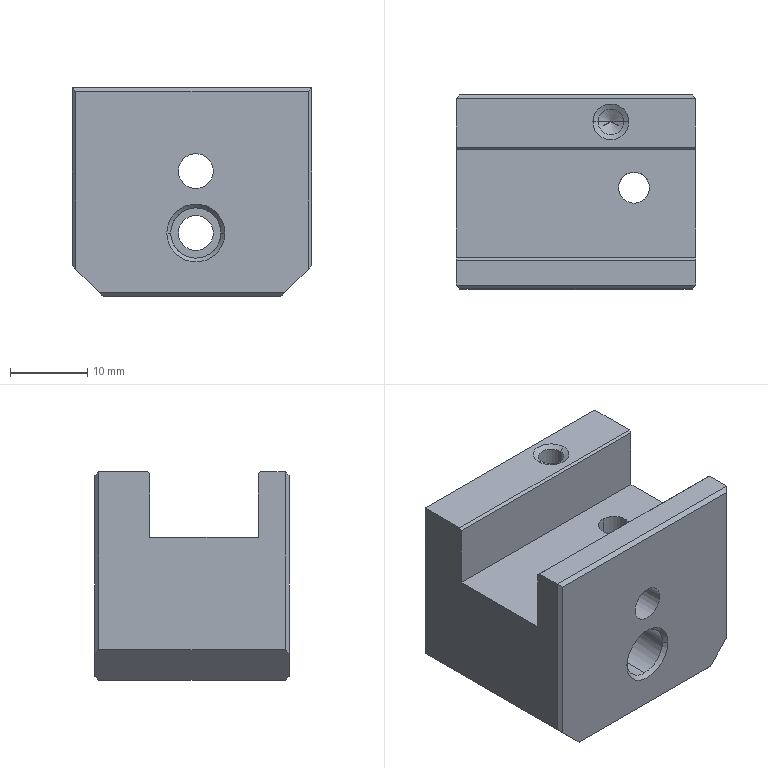Part | NX | 1 solid | 51 faces | box 31 x 25.1 x 27 mm | volume 15480 mm3 | plane 23 | cone 14 | cylinder 14 | commonest cylinder face diameters 3.3 x6 4.5 x4 4 x2 6.5 x2
STEP:
#1=CARTESIAN_POINT('',(29.,6.2,0.));
#2=VERTEX_POINT('',#1);
#3=CARTESIAN_POINT('',(-2.,6.2,0.));
#4=VERTEX_POINT('',#3);
#5=CARTESIAN_POINT('',(0.,6.2,0.));
#6=DIRECTION('',(-1.,0.,0.));
#7=VECTOR('',#6,1000.);
#8=LINE('',#5,#7);
#9=EDGE_CURVE('',#2,#4,#8,.T.);
#10=ORIENTED_EDGE('',*,*,#9,.T.);
#11=CARTESIAN_POINT('',(-2.,3.,0.));
#12=VERTEX_POINT('',#11);
#13=CARTESIAN_POINT('',(-2.,0.,0.));
#14=DIRECTION('',(0.,1.,0.));
#15=VECTOR('',#14,1000.);
#16=LINE('',#13,#15);
#17=EDGE_CURVE('',#12,#4,#16,.T.);
#18=ORIENTED_EDGE('',*,*,#17,.F.);
#19=CARTESIAN_POINT('',(29.,3.,0.));
#20=VERTEX_POINT('',#19);
#21=CARTESIAN_POINT('',(0.,3.,0.));
#22=DIRECTION('',(1.,0.,0.));
#23=VECTOR('',#22,1000.);
#24=LINE('',#21,#23);
#25=EDGE_CURVE('',#12,#20,#24,.T.);
#26=ORIENTED_EDGE('',*,*,#25,.T.);
#27=CARTESIAN_POINT('',(29.,0.,0.));
#28=DIRECTION('',(0.,-1.,0.));
#29=VECTOR('',#28,1000.);
#30=LINE('',#27,#29);
#31=EDGE_CURVE('',#2,#20,#30,.T.);
#32=ORIENTED_EDGE('',*,*,#31,.F.);
#33=EDGE_LOOP('',(#10,#18,#26,#32));
#34=FACE_BOUND('',#33,.T.);
#35=CARTESIAN_POINT('',(0.,0.,0.));
#36=DIRECTION('',(0.,0.,1.));
#37=DIRECTION('',(1.,0.,0.));
#38=AXIS2_PLACEMENT_3D('',#35,#36,#37);
#39=PLANE('',#38);
#40=ADVANCED_FACE('',(#34),#39,.T.);
#41=CARTESIAN_POINT('',(29.,6.5,-0.3));
#42=VERTEX_POINT('',#41);
#43=CARTESIAN_POINT('',(-2.,6.5,-0.3));
#44=VERTEX_POINT('',#43);
#45=CARTESIAN_POINT('',(0.,6.5,-0.3));
#46=DIRECTION('',(-1.,0.,0.));
#47=VECTOR('',#46,1000.);
#48=LINE('',#45,#47);
#49=EDGE_CURVE('',#42,#44,#48,.T.);
#50=ORIENTED_EDGE('',*,*,#49,.F.);
#51=CARTESIAN_POINT('',(29.,6.5,-8.5));
#52=VERTEX_POINT('',#51);
#53=CARTESIAN_POINT('',(29.,6.5,0.));
#54=DIRECTION('',(0.,0.,-1.));
#55=VECTOR('',#54,1000.);
#56=LINE('',#53,#55);
#57=EDGE_CURVE('',#42,#52,#56,.T.);
#58=ORIENTED_EDGE('',*,*,#57,.T.);
#59=CARTESIAN_POINT('',(-2.,6.5,-8.5));
#60=VERTEX_POINT('',#59);
#61=CARTESIAN_POINT('',(0.,6.5,-8.5));
#62=DIRECTION('',(1.,0.,0.));
#63=VECTOR('',#62,1000.);
#64=LINE('',#61,#63);
#65=EDGE_CURVE('',#60,#52,#64,.T.);
#66=ORIENTED_EDGE('',*,*,#65,.F.);
#67=CARTESIAN_POINT('',(-2.,6.5,0.));
#68=DIRECTION('',(0.,0.,1.));
#69=VECTOR('',#68,1000.);
#70=LINE('',#67,#69);
#71=EDGE_CURVE('',#60,#44,#70,.T.);
#72=ORIENTED_EDGE('',*,*,#71,.T.);
#73=EDGE_LOOP('',(#50,#58,#66,#72));
#74=FACE_BOUND('',#73,.T.);
#75=CARTESIAN_POINT('',(30.,6.5,0.));
#76=DIRECTION('',(0.,-1.,0.));
#77=DIRECTION('',(0.,0.,-1.));
#78=AXIS2_PLACEMENT_3D('',#75,#76,#77);
#79=PLANE('',#78);
#80=ADVANCED_FACE('',(#74),#79,.F.);
#81=CARTESIAN_POINT('',(29.,3.,-23.));
#82=VERTEX_POINT('',#81);
#83=CARTESIAN_POINT('',(29.,27.1,-23.));
#84=VERTEX_POINT('',#83);
#85=CARTESIAN_POINT('',(29.,0.,-23.));
#86=DIRECTION('',(0.,1.,0.));
#87=VECTOR('',#86,1000.);
#88=LINE('',#85,#87);
#89=EDGE_CURVE('',#82,#84,#88,.T.);
#90=ORIENTED_EDGE('',*,*,#89,.T.);
#91=CARTESIAN_POINT('',(29.,27.1,0.));
#92=VERTEX_POINT('',#91);
#93=CARTESIAN_POINT('',(29.,27.1,0.));
#94=DIRECTION('',(0.,0.,1.));
#95=VECTOR('',#94,1000.);
#96=LINE('',#93,#95);
#97=EDGE_CURVE('',#84,#92,#96,.T.);
#98=ORIENTED_EDGE('',*,*,#97,.T.);
#99=CARTESIAN_POINT('',(29.,20.8,0.));
#100=VERTEX_POINT('',#99);
#101=CARTESIAN_POINT('',(29.,0.,0.));
#102=DIRECTION('',(0.,-1.,0.));
#103=VECTOR('',#102,1000.);
#104=LINE('',#101,#103);
#105=EDGE_CURVE('',#92,#100,#104,.T.);
#106=ORIENTED_EDGE('',*,*,#105,.T.);
#107=CARTESIAN_POINT('',(29.,20.5,-0.3));
#108=VERTEX_POINT('',#107);
#109=CARTESIAN_POINT('',(29.,20.8,0.));
#110=DIRECTION('',(0.,-0.7071,-0.7071));
#111=VECTOR('',#110,1000.);
#112=LINE('',#109,#111);
#113=EDGE_CURVE('',#100,#108,#112,.T.);
#114=ORIENTED_EDGE('',*,*,#113,.T.);
#115=CARTESIAN_POINT('',(29.,20.5,-8.5));
#116=VERTEX_POINT('',#115);
#117=CARTESIAN_POINT('',(29.,20.5,0.));
#118=DIRECTION('',(0.,0.,1.));
#119=VECTOR('',#118,1000.);
#120=LINE('',#117,#119);
#121=EDGE_CURVE('',#116,#108,#120,.T.);
#122=ORIENTED_EDGE('',*,*,#121,.F.);
#123=CARTESIAN_POINT('',(29.,0.,-8.5));
#124=DIRECTION('',(0.,1.,0.));
#125=VECTOR('',#124,1000.);
#126=LINE('',#123,#125);
#127=EDGE_CURVE('',#52,#116,#126,.T.);
#128=ORIENTED_EDGE('',*,*,#127,.F.);
#129=ORIENTED_EDGE('',*,*,#57,.F.);
#130=CARTESIAN_POINT('',(29.,6.2,0.));
#131=DIRECTION('',(0.,-0.7071,0.7071));
#132=VECTOR('',#131,1000.);
#133=LINE('',#130,#132);
#134=EDGE_CURVE('',#42,#2,#133,.T.);
#135=ORIENTED_EDGE('',*,*,#134,.T.);
#136=ORIENTED_EDGE('',*,*,#31,.T.);
#137=CARTESIAN_POINT('',(29.,3.,0.));
#138=DIRECTION('',(0.,0.,1.));
#139=VECTOR('',#138,1000.);
#140=LINE('',#137,#139);
#141=EDGE_CURVE('',#82,#20,#140,.T.);
#142=ORIENTED_EDGE('',*,*,#141,.F.);
#143=EDGE_LOOP('',(#90,#98,#106,#114,#122,#128,#129,#135,#136,#142));
#144=FACE_BOUND('',#143,.T.);
#145=CARTESIAN_POINT('',(29.,7.685,-15.));
#146=VERTEX_POINT('',#145);
#147=CARTESIAN_POINT('',(29.,12.315,-15.));
#148=VERTEX_POINT('',#147);
#149=CARTESIAN_POINT('',(29.,10.,-15.));
#150=DIRECTION('',(1.,0.,0.));
#151=DIRECTION('',(0.,-1.,0.));
#152=AXIS2_PLACEMENT_3D('',#149,#150,#151);
#153=CIRCLE('',#152,2.315);
#154=EDGE_CURVE('',#146,#148,#153,.T.);
#155=ORIENTED_EDGE('',*,*,#154,.F.);
#156=CARTESIAN_POINT('',(29.,10.,-15.));
#157=DIRECTION('',(1.,0.,0.));
#158=DIRECTION('',(0.,-1.,0.));
#159=AXIS2_PLACEMENT_3D('',#156,#157,#158);
#160=CIRCLE('',#159,2.315);
#161=EDGE_CURVE('',#148,#146,#160,.T.);
#162=ORIENTED_EDGE('',*,*,#161,.F.);
#163=EDGE_LOOP('',(#155,#162));
#164=FACE_BOUND('',#163,.T.);
#165=CARTESIAN_POINT('',(29.,0.,0.));
#166=DIRECTION('',(1.,0.,0.));
#167=DIRECTION('',(0.,1.,0.));
#168=AXIS2_PLACEMENT_3D('',#165,#166,#167);
#169=PLANE('',#168);
#170=ADVANCED_FACE('',(#144,#164),#169,.T.);
#171=ORIENTED_EDGE('',*,*,#127,.T.);
#172=CARTESIAN_POINT('',(-2.,20.5,-8.5));
#173=VERTEX_POINT('',#172);
#174=CARTESIAN_POINT('',(0.,20.5,-8.5));
#175=DIRECTION('',(1.,0.,0.));
#176=VECTOR('',#175,1000.);
#177=LINE('',#174,#176);
#178=EDGE_CURVE('',#173,#116,#177,.T.);
#179=ORIENTED_EDGE('',*,*,#178,.F.);
#180=CARTESIAN_POINT('',(-2.,0.,-8.5));
#181=DIRECTION('',(0.,-1.,0.));
#182=VECTOR('',#181,1000.);
#183=LINE('',#180,#182);
#184=EDGE_CURVE('',#173,#60,#183,.T.);
#185=ORIENTED_EDGE('',*,*,#184,.T.);
#186=ORIENTED_EDGE('',*,*,#65,.T.);
#187=EDGE_LOOP('',(#171,#179,#185,#186));
#188=FACE_BOUND('',#187,.T.);
#189=CARTESIAN_POINT('',(21.,17.6,-8.5));
#190=VERTEX_POINT('',#189);
#191=CARTESIAN_POINT('',(21.,13.6,-8.5));
#192=VERTEX_POINT('',#191);
#193=CARTESIAN_POINT('',(21.,15.6,-8.5));
#194=DIRECTION('',(0.,0.,-1.));
#195=DIRECTION('',(0.,-1.,0.));
#196=AXIS2_PLACEMENT_3D('',#193,#194,#195);
#197=CIRCLE('',#196,2.);
#198=EDGE_CURVE('',#190,#192,#197,.T.);
#199=ORIENTED_EDGE('',*,*,#198,.T.);
#200=CARTESIAN_POINT('',(21.,15.6,-8.5));
#201=DIRECTION('',(0.,0.,-1.));
#202=DIRECTION('',(0.,-1.,0.));
#203=AXIS2_PLACEMENT_3D('',#200,#201,#202);
#204=CIRCLE('',#203,2.);
#205=EDGE_CURVE('',#192,#190,#204,.T.);
#206=ORIENTED_EDGE('',*,*,#205,.T.);
#207=EDGE_LOOP('',(#199,#206));
#208=FACE_BOUND('',#207,.T.);
#209=CARTESIAN_POINT('',(30.,6.5,-8.5));
#210=DIRECTION('',(0.,0.,-1.));
#211=DIRECTION('',(0.,-1.,0.));
#212=AXIS2_PLACEMENT_3D('',#209,#210,#211);
#213=PLANE('',#212);
#214=ADVANCED_FACE('',(#188,#208),#213,.F.);
#215=CARTESIAN_POINT('',(17.75,2.5,-18.8));
#216=VERTEX_POINT('',#215);
#217=CARTESIAN_POINT('',(10.25,2.5,-18.8));
#218=VERTEX_POINT('',#217);
#219=CARTESIAN_POINT('',(14.,2.5,-18.8));
#220=DIRECTION('',(0.,-1.,0.));
#221=DIRECTION('',(-1.,0.,0.));
#222=AXIS2_PLACEMENT_3D('',#219,#220,#221);
#223=CIRCLE('',#222,3.75);
#224=EDGE_CURVE('',#216,#218,#223,.T.);
#225=ORIENTED_EDGE('',*,*,#224,.T.);
#226=CARTESIAN_POINT('',(10.75,3.,-18.8));
#227=VERTEX_POINT('',#226);
#228=CARTESIAN_POINT('',(10.25,2.5,-18.8));
#229=DIRECTION('',(-0.7071,-0.7071,0.));
#230=VECTOR('',#229,1000.);
#231=LINE('',#228,#230);
#232=EDGE_CURVE('',#218,#227,#231,.F.);
#233=ORIENTED_EDGE('',*,*,#232,.T.);
#234=CARTESIAN_POINT('',(14.,3.,-15.55));
#235=VERTEX_POINT('',#234);
#236=CARTESIAN_POINT('',(14.,3.,-18.8));
#237=DIRECTION('',(0.,-1.,0.));
#238=DIRECTION('',(-1.,0.,0.));
#239=AXIS2_PLACEMENT_3D('',#236,#237,#238);
#240=CIRCLE('',#239,3.25);
#241=EDGE_CURVE('',#235,#227,#240,.T.);
#242=ORIENTED_EDGE('',*,*,#241,.F.);
#243=CARTESIAN_POINT('',(17.25,3.,-18.8));
#244=VERTEX_POINT('',#243);
#245=CARTESIAN_POINT('',(14.,3.,-18.8));
#246=DIRECTION('',(0.,-1.,0.));
#247=DIRECTION('',(-1.,0.,0.));
#248=AXIS2_PLACEMENT_3D('',#245,#246,#247);
#249=CIRCLE('',#248,3.25);
#250=EDGE_CURVE('',#244,#235,#249,.T.);
#251=ORIENTED_EDGE('',*,*,#250,.F.);
#252=CARTESIAN_POINT('',(17.75,2.5,-18.8));
#253=DIRECTION('',(0.7071,-0.7071,0.));
#254=VECTOR('',#253,1000.);
#255=LINE('',#252,#254);
#256=EDGE_CURVE('',#216,#244,#255,.F.);
#257=ORIENTED_EDGE('',*,*,#256,.F.);
#258=EDGE_LOOP('',(#225,#233,#242,#251,#257));
#259=FACE_BOUND('',#258,.T.);
#260=CARTESIAN_POINT('',(14.,2.5,-18.8));
#261=DIRECTION('',(0.,-1.,0.));
#262=DIRECTION('',(-1.,0.,0.));
#263=AXIS2_PLACEMENT_3D('',#260,#261,#262);
#264=CONICAL_SURFACE('',#263,3.75,0.7854);
#265=ADVANCED_FACE('',(#259),#264,.F.);
#266=CARTESIAN_POINT('',(-2.,20.8,0.));
#267=VERTEX_POINT('',#266);
#268=CARTESIAN_POINT('',(0.,20.8,0.));
#269=DIRECTION('',(1.,0.,0.));
#270=VECTOR('',#269,1000.);
#271=LINE('',#268,#270);
#272=EDGE_CURVE('',#267,#100,#271,.T.);
#273=ORIENTED_EDGE('',*,*,#272,.T.);
#274=ORIENTED_EDGE('',*,*,#105,.F.);
#275=CARTESIAN_POINT('',(-2.,27.1,0.));
#276=VERTEX_POINT('',#275);
#277=CARTESIAN_POINT('',(0.,27.1,0.));
#278=DIRECTION('',(1.,0.,0.));
#279=VECTOR('',#278,1000.);
#280=LINE('',#277,#279);
#281=EDGE_CURVE('',#276,#92,#280,.T.);
#282=ORIENTED_EDGE('',*,*,#281,.F.);
#283=CARTESIAN_POINT('',(-2.,0.,0.));
#284=DIRECTION('',(0.,1.,0.));
#285=VECTOR('',#284,1000.);
#286=LINE('',#283,#285);
#287=EDGE_CURVE('',#267,#276,#286,.T.);
#288=ORIENTED_EDGE('',*,*,#287,.F.);
#289=EDGE_LOOP('',(#273,#274,#282,#288));
#290=FACE_BOUND('',#289,.T.);
#291=CARTESIAN_POINT('',(20.315,24.1,0.));
#292=VERTEX_POINT('',#291);
#293=CARTESIAN_POINT('',(15.685,24.1,0.));
#294=VERTEX_POINT('',#293);
#295=CARTESIAN_POINT('',(18.,24.1,0.));
#296=DIRECTION('',(0.,0.,1.));
#297=DIRECTION('',(1.,0.,0.));
#298=AXIS2_PLACEMENT_3D('',#295,#296,#297);
#299=CIRCLE('',#298,2.315);
#300=EDGE_CURVE('',#292,#294,#299,.T.);
#301=ORIENTED_EDGE('',*,*,#300,.F.);
#302=CARTESIAN_POINT('',(18.,24.1,0.));
#303=DIRECTION('',(0.,0.,1.));
#304=DIRECTION('',(1.,0.,0.));
#305=AXIS2_PLACEMENT_3D('',#302,#303,#304);
#306=CIRCLE('',#305,2.315);
#307=EDGE_CURVE('',#294,#292,#306,.T.);
#308=ORIENTED_EDGE('',*,*,#307,.F.);
#309=EDGE_LOOP('',(#301,#308));
#310=FACE_BOUND('',#309,.T.);
#311=CARTESIAN_POINT('',(0.,0.,0.));
#312=DIRECTION('',(0.,0.,1.));
#313=DIRECTION('',(1.,0.,0.));
#314=AXIS2_PLACEMENT_3D('',#311,#312,#313);
#315=PLANE('',#314);
#316=ADVANCED_FACE('',(#290,#310),#315,.T.);
#317=CARTESIAN_POINT('',(-2.,20.5,-0.3));
#318=VERTEX_POINT('',#317);
#319=CARTESIAN_POINT('',(0.,20.5,-0.3));
#320=DIRECTION('',(1.,0.,0.));
#321=VECTOR('',#320,1000.);
#322=LINE('',#319,#321);
#323=EDGE_CURVE('',#318,#108,#322,.T.);
#324=ORIENTED_EDGE('',*,*,#323,.F.);
#325=CARTESIAN_POINT('',(-2.,20.5,0.));
#326=DIRECTION('',(0.,0.,-1.));
#327=VECTOR('',#326,1000.);
#328=LINE('',#325,#327);
#329=EDGE_CURVE('',#318,#173,#328,.T.);
#330=ORIENTED_EDGE('',*,*,#329,.T.);
#331=ORIENTED_EDGE('',*,*,#178,.T.);
#332=ORIENTED_EDGE('',*,*,#121,.T.);
#333=EDGE_LOOP('',(#324,#330,#331,#332));
#334=FACE_BOUND('',#333,.T.);
#335=CARTESIAN_POINT('',(30.,20.5,-8.5));
#336=DIRECTION('',(0.,1.,0.));
#337=DIRECTION('',(1.,0.,0.));
#338=AXIS2_PLACEMENT_3D('',#335,#336,#337);
#339=PLANE('',#338);
#340=ADVANCED_FACE('',(#334),#339,.F.);
#341=CARTESIAN_POINT('',(2.,3.,-27.));
#342=VERTEX_POINT('',#341);
#343=CARTESIAN_POINT('',(2.,27.1,-27.));
#344=VERTEX_POINT('',#343);
#345=CARTESIAN_POINT('',(2.,0.,-27.));
#346=DIRECTION('',(0.,1.,0.));
#347=VECTOR('',#346,1000.);
#348=LINE('',#345,#347);
#349=EDGE_CURVE('',#342,#344,#348,.T.);
#350=ORIENTED_EDGE('',*,*,#349,.T.);
#351=CARTESIAN_POINT('',(25.,27.1,-27.));
#352=VERTEX_POINT('',#351);
#353=CARTESIAN_POINT('',(0.,27.1,-27.));
#354=DIRECTION('',(-1.,0.,0.));
#355=VECTOR('',#354,1000.);
#356=LINE('',#353,#355);
#357=EDGE_CURVE('',#352,#344,#356,.T.);
#358=ORIENTED_EDGE('',*,*,#357,.F.);
#359=CARTESIAN_POINT('',(25.,3.,-27.));
#360=VERTEX_POINT('',#359);
#361=CARTESIAN_POINT('',(25.,0.,-27.));
#362=DIRECTION('',(0.,1.,0.));
#363=VECTOR('',#362,1000.);
#364=LINE('',#361,#363);
#365=EDGE_CURVE('',#360,#352,#364,.T.);
#366=ORIENTED_EDGE('',*,*,#365,.F.);
#367=CARTESIAN_POINT('',(0.,3.,-27.));
#368=DIRECTION('',(1.,0.,0.));
#369=VECTOR('',#368,1000.);
#370=LINE('',#367,#369);
#371=EDGE_CURVE('',#342,#360,#370,.T.);
#372=ORIENTED_EDGE('',*,*,#371,.F.);
#373=EDGE_LOOP('',(#350,#358,#366,#372));
#374=FACE_BOUND('',#373,.T.);
#375=CARTESIAN_POINT('',(10.315,15.6,-27.));
#376=VERTEX_POINT('',#375);
#377=CARTESIAN_POINT('',(5.685,15.6,-27.));
#378=VERTEX_POINT('',#377);
#379=CARTESIAN_POINT('',(8.,15.6,-27.));
#380=DIRECTION('',(0.,0.,-1.));
#381=DIRECTION('',(-1.,0.,0.));
#382=AXIS2_PLACEMENT_3D('',#379,#380,#381);
#383=CIRCLE('',#382,2.315);
#384=EDGE_CURVE('',#376,#378,#383,.T.);
#385=ORIENTED_EDGE('',*,*,#384,.F.);
#386=CARTESIAN_POINT('',(8.,15.6,-27.));
#387=DIRECTION('',(0.,0.,-1.));
#388=DIRECTION('',(-1.,0.,0.));
#389=AXIS2_PLACEMENT_3D('',#386,#387,#388);
#390=CIRCLE('',#389,2.315);
#391=EDGE_CURVE('',#378,#376,#390,.T.);
#392=ORIENTED_EDGE('',*,*,#391,.F.);
#393=EDGE_LOOP('',(#385,#392));
#394=FACE_BOUND('',#393,.T.);
#395=CARTESIAN_POINT('',(21.,13.6,-27.));
#396=VERTEX_POINT('',#395);
#397=CARTESIAN_POINT('',(21.,17.6,-27.));
#398=VERTEX_POINT('',#397);
#399=CARTESIAN_POINT('',(21.,15.6,-27.));
#400=DIRECTION('',(0.,0.,-1.));
#401=DIRECTION('',(0.,-1.,0.));
#402=AXIS2_PLACEMENT_3D('',#399,#400,#401);
#403=CIRCLE('',#402,2.);
#404=EDGE_CURVE('',#396,#398,#403,.T.);
#405=ORIENTED_EDGE('',*,*,#404,.F.);
#406=CARTESIAN_POINT('',(21.,15.6,-27.));
#407=DIRECTION('',(0.,0.,-1.));
#408=DIRECTION('',(0.,-1.,0.));
#409=AXIS2_PLACEMENT_3D('',#406,#407,#408);
#410=CIRCLE('',#409,2.);
#411=EDGE_CURVE('',#398,#396,#410,.T.);
#412=ORIENTED_EDGE('',*,*,#411,.F.);
#413=EDGE_LOOP('',(#405,#412));
#414=FACE_BOUND('',#413,.T.);
#415=CARTESIAN_POINT('',(0.,0.,-27.));
#416=DIRECTION('',(0.,0.,1.));
#417=DIRECTION('',(1.,0.,0.));
#418=AXIS2_PLACEMENT_3D('',#415,#416,#417);
#419=PLANE('',#418);
#420=ADVANCED_FACE('',(#374,#394,#414),#419,.F.);
#421=CARTESIAN_POINT('',(-2.,3.,-23.));
#422=VERTEX_POINT('',#421);
#423=CARTESIAN_POINT('',(-2.,3.,0.));
#424=DIRECTION('',(0.,0.,1.));
#425=VECTOR('',#424,1000.);
#426=LINE('',#423,#425);
#427=EDGE_CURVE('',#422,#12,#426,.T.);
#428=ORIENTED_EDGE('',*,*,#427,.T.);
#429=ORIENTED_EDGE('',*,*,#17,.T.);
#430=CARTESIAN_POINT('',(-2.,6.2,0.));
#431=DIRECTION('',(0.,0.7071,-0.7071));
#432=VECTOR('',#431,1000.);
#433=LINE('',#430,#432);
#434=EDGE_CURVE('',#4,#44,#433,.T.);
#435=ORIENTED_EDGE('',*,*,#434,.T.);
#436=ORIENTED_EDGE('',*,*,#71,.F.);
#437=ORIENTED_EDGE('',*,*,#184,.F.);
#438=ORIENTED_EDGE('',*,*,#329,.F.);
#439=CARTESIAN_POINT('',(-2.,20.8,0.));
#440=DIRECTION('',(0.,0.7071,0.7071));
#441=VECTOR('',#440,1000.);
#442=LINE('',#439,#441);
#443=EDGE_CURVE('',#318,#267,#442,.T.);
#444=ORIENTED_EDGE('',*,*,#443,.T.);
#445=ORIENTED_EDGE('',*,*,#287,.T.);
#446=CARTESIAN_POINT('',(-2.,27.1,-23.));
#447=VERTEX_POINT('',#446);
#448=CARTESIAN_POINT('',(-2.,27.1,0.));
#449=DIRECTION('',(0.,0.,-1.));
#450=VECTOR('',#449,1000.);
#451=LINE('',#448,#450);
#452=EDGE_CURVE('',#276,#447,#451,.T.);
#453=ORIENTED_EDGE('',*,*,#452,.T.);
#454=CARTESIAN_POINT('',(-2.,0.,-23.));
#455=DIRECTION('',(0.,1.,0.));
#456=VECTOR('',#455,1000.);
#457=LINE('',#454,#456);
#458=EDGE_CURVE('',#422,#447,#457,.T.);
#459=ORIENTED_EDGE('',*,*,#458,.F.);
#460=EDGE_LOOP('',(#428,#429,#435,#436,#437,#438,#444,#445,#453,#459));
#461=FACE_BOUND('',#460,.T.);
#462=CARTESIAN_POINT('',(-2.,27.6,0.));
#463=DIRECTION('',(-1.,0.,0.));
#464=DIRECTION('',(0.,0.,1.));
#465=AXIS2_PLACEMENT_3D('',#462,#463,#464);
#466=PLANE('',#465);
#467=ADVANCED_FACE('',(#461),#466,.T.);
#468=CARTESIAN_POINT('',(14.,7.5,-15.55));
#469=VERTEX_POINT('',#468);
#470=CARTESIAN_POINT('',(14.,7.5,-22.05));
#471=VERTEX_POINT('',#470);
#472=CARTESIAN_POINT('',(14.,7.5,-18.8));
#473=DIRECTION('',(0.,-1.,0.));
#474=DIRECTION('',(0.,0.,1.));
#475=AXIS2_PLACEMENT_3D('',#472,#473,#474);
#476=CIRCLE('',#475,3.25);
#477=EDGE_CURVE('',#469,#471,#476,.T.);
#478=ORIENTED_EDGE('',*,*,#477,.T.);
#479=CARTESIAN_POINT('',(14.,7.5,-18.8));
#480=DIRECTION('',(0.,-1.,0.));
#481=DIRECTION('',(0.,0.,1.));
#482=AXIS2_PLACEMENT_3D('',#479,#480,#481);
#483=CIRCLE('',#482,3.25);
#484=EDGE_CURVE('',#471,#469,#483,.T.);
#485=ORIENTED_EDGE('',*,*,#484,.T.);
#486=EDGE_LOOP('',(#478,#485));
#487=FACE_BOUND('',#486,.T.);
#488=CARTESIAN_POINT('',(11.75,7.5,-18.8));
#489=VERTEX_POINT('',#488);
#490=CARTESIAN_POINT('',(16.25,7.5,-18.8));
#491=VERTEX_POINT('',#490);
#492=CARTESIAN_POINT('',(14.,7.5,-18.8));
#493=DIRECTION('',(0.,-1.,0.));
#494=DIRECTION('',(1.,0.,0.));
#495=AXIS2_PLACEMENT_3D('',#492,#493,#494);
#496=CIRCLE('',#495,2.25);
#497=EDGE_CURVE('',#489,#491,#496,.T.);
#498=ORIENTED_EDGE('',*,*,#497,.F.);
#499=CARTESIAN_POINT('',(14.,7.5,-18.8));
#500=DIRECTION('',(0.,-1.,0.));
#501=DIRECTION('',(1.,0.,0.));
#502=AXIS2_PLACEMENT_3D('',#499,#500,#501);
#503=CIRCLE('',#502,2.25);
#504=EDGE_CURVE('',#491,#489,#503,.T.);
#505=ORIENTED_EDGE('',*,*,#504,.F.);
#506=EDGE_LOOP('',(#498,#505));
#507=FACE_BOUND('',#506,.T.);
#508=CARTESIAN_POINT('',(24.886,7.5,-17.71));
#509=DIRECTION('',(0.,-1.,0.));
#510=DIRECTION('',(0.,0.,-1.));
#511=AXIS2_PLACEMENT_3D('',#508,#509,#510);
#512=PLANE('',#511);
#513=ADVANCED_FACE('',(#487,#507),#512,.T.);
#514=CARTESIAN_POINT('',(16.25,27.6,-10.8));
#515=VERTEX_POINT('',#514);
#516=CARTESIAN_POINT('',(11.75,27.6,-10.8));
#517=VERTEX_POINT('',#516);
#518=CARTESIAN_POINT('',(14.,27.6,-10.8));
#519=DIRECTION('',(0.,-1.,0.));
#520=DIRECTION('',(1.,0.,0.));
#521=AXIS2_PLACEMENT_3D('',#518,#519,#520);
#522=CIRCLE('',#521,2.25);
#523=EDGE_CURVE('',#515,#517,#522,.T.);
#524=ORIENTED_EDGE('',*,*,#523,.F.);
#525=CARTESIAN_POINT('',(16.25,2.5,-10.8));
#526=VERTEX_POINT('',#525);
#527=CARTESIAN_POINT('',(16.25,27.6,-10.8));
#528=DIRECTION('',(0.,-1.,0.));
#529=VECTOR('',#528,1000.);
#530=LINE('',#527,#529);
#531=EDGE_CURVE('',#515,#526,#530,.T.);
#532=ORIENTED_EDGE('',*,*,#531,.T.);
#533=CARTESIAN_POINT('',(11.75,2.5,-10.8));
#534=VERTEX_POINT('',#533);
#535=CARTESIAN_POINT('',(14.,2.5,-10.8));
#536=DIRECTION('',(0.,-1.,0.));
#537=DIRECTION('',(1.,0.,0.));
#538=AXIS2_PLACEMENT_3D('',#535,#536,#537);
#539=CIRCLE('',#538,2.25);
#540=EDGE_CURVE('',#526,#534,#539,.T.);
#541=ORIENTED_EDGE('',*,*,#540,.T.);
#542=CARTESIAN_POINT('',(11.75,27.6,-10.8));
#543=DIRECTION('',(0.,-1.,0.));
#544=VECTOR('',#543,1000.);
#545=LINE('',#542,#544);
#546=EDGE_CURVE('',#517,#534,#545,.T.);
#547=ORIENTED_EDGE('',*,*,#546,.F.);
#548=EDGE_LOOP('',(#524,#532,#541,#547));
#549=FACE_BOUND('',#548,.T.);
#550=CARTESIAN_POINT('',(14.,27.6,-10.8));
#551=DIRECTION('',(0.,-1.,0.));
#552=DIRECTION('',(1.,0.,0.));
#553=AXIS2_PLACEMENT_3D('',#550,#551,#552);
#554=CYLINDRICAL_SURFACE('',#553,2.25);
#555=ADVANCED_FACE('',(#549),#554,.F.);
#556=CARTESIAN_POINT('',(-1.5,27.6,-23.5));
#557=VERTEX_POINT('',#556);
#558=CARTESIAN_POINT('',(-1.5,27.6,-0.5));
#559=VERTEX_POINT('',#558);
#560=CARTESIAN_POINT('',(-1.5,27.6,0.));
#561=DIRECTION('',(0.,0.,1.));
#562=VECTOR('',#561,1000.);
#563=LINE('',#560,#562);
#564=EDGE_CURVE('',#557,#559,#563,.T.);
#565=ORIENTED_EDGE('',*,*,#564,.T.);
#566=CARTESIAN_POINT('',(28.5,27.6,-0.5));
#567=VERTEX_POINT('',#566);
#568=CARTESIAN_POINT('',(0.,27.6,-0.5));
#569=DIRECTION('',(-1.,0.,0.));
#570=VECTOR('',#569,1000.);
#571=LINE('',#568,#570);
#572=EDGE_CURVE('',#567,#559,#571,.T.);
#573=ORIENTED_EDGE('',*,*,#572,.F.);
#574=CARTESIAN_POINT('',(28.5,27.6,-23.5));
#575=VERTEX_POINT('',#574);
#576=CARTESIAN_POINT('',(28.5,27.6,0.));
#577=DIRECTION('',(0.,0.,-1.));
#578=VECTOR('',#577,1000.);
#579=LINE('',#576,#578);
#580=EDGE_CURVE('',#567,#575,#579,.T.);
#581=ORIENTED_EDGE('',*,*,#580,.T.);
#582=CARTESIAN_POINT('',(25.5,27.6,-26.5));
#583=VERTEX_POINT('',#582);
#584=CARTESIAN_POINT('',(52.,27.6,0.));
#585=DIRECTION('',(-0.7071,0.,-0.7071));
#586=VECTOR('',#585,1000.);
#587=LINE('',#584,#586);
#588=EDGE_CURVE('',#575,#583,#587,.T.);
#589=ORIENTED_EDGE('',*,*,#588,.T.);
#590=CARTESIAN_POINT('',(1.5,27.6,-26.5));
#591=VERTEX_POINT('',#590);
#592=CARTESIAN_POINT('',(0.,27.6,-26.5));
#593=DIRECTION('',(-1.,0.,0.));
#594=VECTOR('',#593,1000.);
#595=LINE('',#592,#594);
#596=EDGE_CURVE('',#583,#591,#595,.T.);
#597=ORIENTED_EDGE('',*,*,#596,.T.);
#598=CARTESIAN_POINT('',(-25.,27.6,0.));
#599=DIRECTION('',(0.7071,0.,-0.7071));
#600=VECTOR('',#599,1000.);
#601=LINE('',#598,#600);
#602=EDGE_CURVE('',#557,#591,#601,.T.);
#603=ORIENTED_EDGE('',*,*,#602,.F.);
#604=EDGE_LOOP('',(#565,#573,#581,#589,#597,#603));
#605=FACE_BOUND('',#604,.T.);
#606=CARTESIAN_POINT('',(11.75,27.6,-18.8));
#607=VERTEX_POINT('',#606);
#608=CARTESIAN_POINT('',(16.25,27.6,-18.8));
#609=VERTEX_POINT('',#608);
#610=CARTESIAN_POINT('',(14.,27.6,-18.8));
#611=DIRECTION('',(0.,-1.,0.));
#612=DIRECTION('',(1.,0.,0.));
#613=AXIS2_PLACEMENT_3D('',#610,#611,#612);
#614=CIRCLE('',#613,2.25);
#615=EDGE_CURVE('',#607,#609,#614,.T.);
#616=ORIENTED_EDGE('',*,*,#615,.T.);
#617=CARTESIAN_POINT('',(14.,27.6,-18.8));
#618=DIRECTION('',(0.,-1.,0.));
#619=DIRECTION('',(1.,0.,0.));
#620=AXIS2_PLACEMENT_3D('',#617,#618,#619);
#621=CIRCLE('',#620,2.25);
#622=EDGE_CURVE('',#609,#607,#621,.T.);
#623=ORIENTED_EDGE('',*,*,#622,.T.);
#624=EDGE_LOOP('',(#616,#623));
#625=FACE_BOUND('',#624,.T.);
#626=ORIENTED_EDGE('',*,*,#523,.T.);
#627=CARTESIAN_POINT('',(14.,27.6,-10.8));
#628=DIRECTION('',(0.,-1.,0.));
#629=DIRECTION('',(1.,0.,0.));
#630=AXIS2_PLACEMENT_3D('',#627,#628,#629);
#631=CIRCLE('',#630,2.25);
#632=EDGE_CURVE('',#517,#515,#631,.T.);
#633=ORIENTED_EDGE('',*,*,#632,.T.);
#634=EDGE_LOOP('',(#626,#633));
#635=FACE_BOUND('',#634,.T.);
#636=CARTESIAN_POINT('',(30.,27.6,0.));
#637=DIRECTION('',(0.,1.,0.));
#638=DIRECTION('',(1.,0.,0.));
#639=AXIS2_PLACEMENT_3D('',#636,#637,#638);
#640=PLANE('',#639);
#641=ADVANCED_FACE('',(#605,#625,#635),#640,.T.);
#642=CARTESIAN_POINT('',(8.,15.6,-13.809));
#643=VERTEX_POINT('',#642);
#644=CARTESIAN_POINT('',(9.65,15.6,-14.8));
#645=VERTEX_POINT('',#644);
#646=CARTESIAN_POINT('',(9.65,15.6,-14.8));
#647=DIRECTION('',(0.8572,0.,-0.515));
#648=VECTOR('',#647,1000.);
#649=LINE('',#646,#648);
#650=EDGE_CURVE('',#643,#645,#649,.T.);
#651=ORIENTED_EDGE('',*,*,#650,.T.);
#652=CARTESIAN_POINT('',(6.35,15.6,-14.8));
#653=VERTEX_POINT('',#652);
#654=CARTESIAN_POINT('',(8.,15.6,-14.8));
#655=DIRECTION('',(0.,0.,-1.));
#656=DIRECTION('',(-1.,0.,0.));
#657=AXIS2_PLACEMENT_3D('',#654,#655,#656);
#658=CIRCLE('',#657,1.65);
#659=EDGE_CURVE('',#645,#653,#658,.T.);
#660=ORIENTED_EDGE('',*,*,#659,.T.);
#661=CARTESIAN_POINT('',(6.35,15.6,-14.8));
#662=DIRECTION('',(-0.8572,0.,-0.515));
#663=VECTOR('',#662,1000.);
#664=LINE('',#661,#663);
#665=EDGE_CURVE('',#643,#653,#664,.T.);
#666=ORIENTED_EDGE('',*,*,#665,.F.);
#667=EDGE_LOOP('',(#651,#660,#666));
#668=FACE_BOUND('',#667,.T.);
#669=CARTESIAN_POINT('',(8.,15.6,-14.8));
#670=DIRECTION('',(0.,0.,-1.));
#671=DIRECTION('',(-1.,0.,0.));
#672=AXIS2_PLACEMENT_3D('',#669,#670,#671);
#673=CONICAL_SURFACE('',#672,1.65,1.03);
#674=ADVANCED_FACE('',(#668),#673,.F.);
#675=ORIENTED_EDGE('',*,*,#404,.T.);
#676=CARTESIAN_POINT('',(21.,17.6,2.7));
#677=DIRECTION('',(0.,0.,-1.));
#678=VECTOR('',#677,1000.);
#679=LINE('',#676,#678);
#680=EDGE_CURVE('',#190,#398,#679,.T.);
#681=ORIENTED_EDGE('',*,*,#680,.F.);
#682=ORIENTED_EDGE('',*,*,#205,.F.);
#683=CARTESIAN_POINT('',(21.,13.6,2.7));
#684=DIRECTION('',(0.,0.,-1.));
#685=VECTOR('',#684,1000.);
#686=LINE('',#683,#685);
#687=EDGE_CURVE('',#192,#396,#686,.T.);
#688=ORIENTED_EDGE('',*,*,#687,.T.);
#689=EDGE_LOOP('',(#675,#681,#682,#688));
#690=FACE_BOUND('',#689,.T.);
#691=CARTESIAN_POINT('',(21.,15.6,2.7));
#692=DIRECTION('',(0.,0.,-1.));
#693=DIRECTION('',(0.,-1.,0.));
#694=AXIS2_PLACEMENT_3D('',#691,#692,#693);
#695=CYLINDRICAL_SURFACE('',#694,2.);
#696=ADVANCED_FACE('',(#690),#695,.F.);
#697=ORIENTED_EDGE('',*,*,#497,.T.);
#698=CARTESIAN_POINT('',(16.25,27.6,-18.8));
#699=DIRECTION('',(0.,-1.,0.));
#700=VECTOR('',#699,1000.);
#701=LINE('',#698,#700);
#702=EDGE_CURVE('',#609,#491,#701,.T.);
#703=ORIENTED_EDGE('',*,*,#702,.F.);
#704=ORIENTED_EDGE('',*,*,#615,.F.);
#705=CARTESIAN_POINT('',(11.75,27.6,-18.8));
#706=DIRECTION('',(0.,-1.,0.));
#707=VECTOR('',#706,1000.);
#708=LINE('',#705,#707);
#709=EDGE_CURVE('',#607,#489,#708,.T.);
#710=ORIENTED_EDGE('',*,*,#709,.T.);
#711=EDGE_LOOP('',(#697,#703,#704,#710));
#712=FACE_BOUND('',#711,.T.);
#713=CARTESIAN_POINT('',(14.,27.6,-18.8));
#714=DIRECTION('',(0.,-1.,0.));
#715=DIRECTION('',(1.,0.,0.));
#716=AXIS2_PLACEMENT_3D('',#713,#714,#715);
#717=CYLINDRICAL_SURFACE('',#716,2.25);
#718=ADVANCED_FACE('',(#712),#717,.F.);
#719=ORIENTED_EDGE('',*,*,#384,.T.);
#720=CARTESIAN_POINT('',(6.35,15.6,-26.616));
#721=VERTEX_POINT('',#720);
#722=CARTESIAN_POINT('',(6.35,15.6,-26.616));
#723=DIRECTION('',(-0.866,0.,-0.5));
#724=VECTOR('',#723,1000.);
#725=LINE('',#722,#724);
#726=EDGE_CURVE('',#378,#721,#725,.F.);
#727=ORIENTED_EDGE('',*,*,#726,.T.);
#728=CARTESIAN_POINT('',(9.65,15.6,-26.616));
#729=VERTEX_POINT('',#728);
#730=CARTESIAN_POINT('',(8.,15.6,-26.616));
#731=DIRECTION('',(0.,0.,-1.));
#732=DIRECTION('',(-1.,0.,0.));
#733=AXIS2_PLACEMENT_3D('',#730,#731,#732);
#734=CIRCLE('',#733,1.65);
#735=EDGE_CURVE('',#729,#721,#734,.T.);
#736=ORIENTED_EDGE('',*,*,#735,.F.);
#737=CARTESIAN_POINT('',(9.65,15.6,-26.616));
#738=DIRECTION('',(0.866,0.,-0.5));
#739=VECTOR('',#738,1000.);
#740=LINE('',#737,#739);
#741=EDGE_CURVE('',#376,#729,#740,.F.);
#742=ORIENTED_EDGE('',*,*,#741,.F.);
#743=EDGE_LOOP('',(#719,#727,#736,#742));
#744=FACE_BOUND('',#743,.T.);
#745=CARTESIAN_POINT('',(8.,15.6,-26.616));
#746=DIRECTION('',(0.,0.,-1.));
#747=DIRECTION('',(-1.,0.,0.));
#748=AXIS2_PLACEMENT_3D('',#745,#746,#747);
#749=CONICAL_SURFACE('',#748,1.65,1.047);
#750=ADVANCED_FACE('',(#744),#749,.F.);
#751=ORIENTED_EDGE('',*,*,#272,.F.);
#752=ORIENTED_EDGE('',*,*,#443,.F.);
#753=ORIENTED_EDGE('',*,*,#323,.T.);
#754=ORIENTED_EDGE('',*,*,#113,.F.);
#755=EDGE_LOOP('',(#751,#752,#753,#754));
#756=FACE_BOUND('',#755,.T.);
#757=CARTESIAN_POINT('',(13.5,20.65,-0.15));
#758=DIRECTION('',(0.,0.7071,-0.7071));
#759=DIRECTION('',(-1.,0.,0.));
#760=AXIS2_PLACEMENT_3D('',#757,#758,#759);
#761=PLANE('',#760);
#762=ADVANCED_FACE('',(#756),#761,.F.);
#763=CARTESIAN_POINT('',(8.,15.6,-26.616));
#764=DIRECTION('',(0.,0.,-1.));
#765=DIRECTION('',(-1.,0.,0.));
#766=AXIS2_PLACEMENT_3D('',#763,#764,#765);
#767=CIRCLE('',#766,1.65);
#768=EDGE_CURVE('',#721,#729,#767,.T.);
#769=ORIENTED_EDGE('',*,*,#768,.T.);
#770=CARTESIAN_POINT('',(9.65,15.6,-27.));
#771=DIRECTION('',(0.,0.,-1.));
#772=VECTOR('',#771,1000.);
#773=LINE('',#770,#772);
#774=EDGE_CURVE('',#645,#729,#773,.T.);
#775=ORIENTED_EDGE('',*,*,#774,.F.);
#776=CARTESIAN_POINT('',(8.,15.6,-14.8));
#777=DIRECTION('',(0.,0.,-1.));
#778=DIRECTION('',(-1.,0.,0.));
#779=AXIS2_PLACEMENT_3D('',#776,#777,#778);
#780=CIRCLE('',#779,1.65);
#781=EDGE_CURVE('',#653,#645,#780,.T.);
#782=ORIENTED_EDGE('',*,*,#781,.F.);
#783=CARTESIAN_POINT('',(6.35,15.6,-27.));
#784=DIRECTION('',(0.,0.,-1.));
#785=VECTOR('',#784,1000.);
#786=LINE('',#783,#785);
#787=EDGE_CURVE('',#653,#721,#786,.T.);
#788=ORIENTED_EDGE('',*,*,#787,.T.);
#789=EDGE_LOOP('',(#769,#775,#782,#788));
#790=FACE_BOUND('',#789,.T.);
#791=CARTESIAN_POINT('',(8.,15.6,-27.));
#792=DIRECTION('',(0.,0.,-1.));
#793=DIRECTION('',(-1.,0.,0.));
#794=AXIS2_PLACEMENT_3D('',#791,#792,#793);
#795=CYLINDRICAL_SURFACE('',#794,1.65);
#796=ADVANCED_FACE('',(#790),#795,.F.);
#797=ORIENTED_EDGE('',*,*,#9,.F.);
#798=ORIENTED_EDGE('',*,*,#134,.F.);
#799=ORIENTED_EDGE('',*,*,#49,.T.);
#800=ORIENTED_EDGE('',*,*,#434,.F.);
#801=EDGE_LOOP('',(#797,#798,#799,#800));
#802=FACE_BOUND('',#801,.T.);
#803=CARTESIAN_POINT('',(13.5,6.35,-0.15));
#804=DIRECTION('',(0.,-0.7071,-0.7071));
#805=DIRECTION('',(0.,0.7071,-0.7071));
#806=AXIS2_PLACEMENT_3D('',#803,#804,#805);
#807=PLANE('',#806);
#808=ADVANCED_FACE('',(#802),#807,.F.);
#809=CARTESIAN_POINT('',(28.616,11.65,-15.));
#810=VERTEX_POINT('',#809);
#811=CARTESIAN_POINT('',(28.616,8.35,-15.));
#812=VERTEX_POINT('',#811);
#813=CARTESIAN_POINT('',(28.616,10.,-15.));
#814=DIRECTION('',(1.,0.,0.));
#815=DIRECTION('',(0.,-1.,0.));
#816=AXIS2_PLACEMENT_3D('',#813,#814,#815);
#817=CIRCLE('',#816,1.65);
#818=EDGE_CURVE('',#810,#812,#817,.T.);
#819=ORIENTED_EDGE('',*,*,#818,.T.);
#820=CARTESIAN_POINT('',(17.8,8.35,-15.));
#821=VERTEX_POINT('',#820);
#822=CARTESIAN_POINT('',(30.,8.35,-15.));
#823=DIRECTION('',(1.,0.,0.));
#824=VECTOR('',#823,1000.);
#825=LINE('',#822,#824);
#826=EDGE_CURVE('',#812,#821,#825,.F.);
#827=ORIENTED_EDGE('',*,*,#826,.T.);
#828=CARTESIAN_POINT('',(17.8,11.65,-15.));
#829=VERTEX_POINT('',#828);
#830=CARTESIAN_POINT('',(17.8,10.,-15.));
#831=DIRECTION('',(1.,0.,0.));
#832=DIRECTION('',(0.,-1.,0.));
#833=AXIS2_PLACEMENT_3D('',#830,#831,#832);
#834=CIRCLE('',#833,1.65);
#835=EDGE_CURVE('',#829,#821,#834,.T.);
#836=ORIENTED_EDGE('',*,*,#835,.F.);
#837=CARTESIAN_POINT('',(30.,11.65,-15.));
#838=DIRECTION('',(1.,0.,0.));
#839=VECTOR('',#838,1000.);
#840=LINE('',#837,#839);
#841=EDGE_CURVE('',#810,#829,#840,.F.);
#842=ORIENTED_EDGE('',*,*,#841,.F.);
#843=EDGE_LOOP('',(#819,#827,#836,#842));
#844=FACE_BOUND('',#843,.T.);
#845=CARTESIAN_POINT('',(30.,10.,-15.));
#846=DIRECTION('',(1.,0.,0.));
#847=DIRECTION('',(0.,-1.,0.));
#848=AXIS2_PLACEMENT_3D('',#845,#846,#847);
#849=CYLINDRICAL_SURFACE('',#848,1.65);
#850=ADVANCED_FACE('',(#844),#849,.F.);
#851=CARTESIAN_POINT('',(16.809,10.,-15.));
#852=VERTEX_POINT('',#851);
#853=CARTESIAN_POINT('',(17.8,11.65,-15.));
#854=DIRECTION('',(0.515,0.8572,0.));
#855=VECTOR('',#854,1000.);
#856=LINE('',#853,#855);
#857=EDGE_CURVE('',#852,#829,#856,.T.);
#858=ORIENTED_EDGE('',*,*,#857,.T.);
#859=ORIENTED_EDGE('',*,*,#835,.T.);
#860=CARTESIAN_POINT('',(17.8,8.35,-15.));
#861=DIRECTION('',(0.515,-0.8572,0.));
#862=VECTOR('',#861,1000.);
#863=LINE('',#860,#862);
#864=EDGE_CURVE('',#852,#821,#863,.T.);
#865=ORIENTED_EDGE('',*,*,#864,.F.);
#866=EDGE_LOOP('',(#858,#859,#865));
#867=FACE_BOUND('',#866,.T.);
#868=CARTESIAN_POINT('',(17.8,10.,-15.));
#869=DIRECTION('',(1.,0.,0.));
#870=DIRECTION('',(0.,-1.,0.));
#871=AXIS2_PLACEMENT_3D('',#868,#869,#870);
#872=CONICAL_SURFACE('',#871,1.65,1.03);
#873=ADVANCED_FACE('',(#867),#872,.F.);
#874=CARTESIAN_POINT('',(1.5,2.5,-26.5));
#875=VERTEX_POINT('',#874);
#876=CARTESIAN_POINT('',(25.5,2.5,-26.5));
#877=VERTEX_POINT('',#876);
#878=CARTESIAN_POINT('',(0.,2.5,-26.5));
#879=DIRECTION('',(1.,0.,0.));
#880=VECTOR('',#879,1000.);
#881=LINE('',#878,#880);
#882=EDGE_CURVE('',#875,#877,#881,.T.);
#883=ORIENTED_EDGE('',*,*,#882,.F.);
#884=CARTESIAN_POINT('',(-25.,-24.,0.));
#885=DIRECTION('',(-0.5774,-0.5774,0.5774));
#886=VECTOR('',#885,1000.);
#887=LINE('',#884,#886);
#888=EDGE_CURVE('',#342,#875,#887,.T.);
#889=ORIENTED_EDGE('',*,*,#888,.F.);
#890=ORIENTED_EDGE('',*,*,#371,.T.);
#891=CARTESIAN_POINT('',(52.,-24.,0.));
#892=DIRECTION('',(0.5774,-0.5774,0.5774));
#893=VECTOR('',#892,1000.);
#894=LINE('',#891,#893);
#895=EDGE_CURVE('',#360,#877,#894,.T.);
#896=ORIENTED_EDGE('',*,*,#895,.T.);
#897=EDGE_LOOP('',(#883,#889,#890,#896));
#898=FACE_BOUND('',#897,.T.);
#899=CARTESIAN_POINT('',(15.,2.75,-26.75));
#900=DIRECTION('',(0.,-0.7071,-0.7071));
#901=DIRECTION('',(0.,-0.7071,0.7071));
#902=AXIS2_PLACEMENT_3D('',#899,#900,#901);
#903=PLANE('',#902);
#904=ADVANCED_FACE('',(#898),#903,.T.);
#905=CARTESIAN_POINT('',(19.65,24.1,-9.));
#906=VERTEX_POINT('',#905);
#907=CARTESIAN_POINT('',(16.35,24.1,-9.));
#908=VERTEX_POINT('',#907);
#909=CARTESIAN_POINT('',(18.,24.1,-9.));
#910=DIRECTION('',(0.,0.,1.));
#911=DIRECTION('',(1.,0.,0.));
#912=AXIS2_PLACEMENT_3D('',#909,#910,#911);
#913=CIRCLE('',#912,1.65);
#914=EDGE_CURVE('',#906,#908,#913,.T.);
#915=ORIENTED_EDGE('',*,*,#914,.F.);
#916=CARTESIAN_POINT('',(19.65,24.1,-0.3839));
#917=VERTEX_POINT('',#916);
#918=CARTESIAN_POINT('',(19.65,24.1,0.));
#919=DIRECTION('',(0.,0.,1.));
#920=VECTOR('',#919,1000.);
#921=LINE('',#918,#920);
#922=EDGE_CURVE('',#906,#917,#921,.T.);
#923=ORIENTED_EDGE('',*,*,#922,.T.);
#924=CARTESIAN_POINT('',(16.35,24.1,-0.3839));
#925=VERTEX_POINT('',#924);
#926=CARTESIAN_POINT('',(18.,24.1,-0.3839));
#927=DIRECTION('',(0.,0.,1.));
#928=DIRECTION('',(1.,0.,0.));
#929=AXIS2_PLACEMENT_3D('',#926,#927,#928);
#930=CIRCLE('',#929,1.65);
#931=EDGE_CURVE('',#917,#925,#930,.T.);
#932=ORIENTED_EDGE('',*,*,#931,.T.);
#933=CARTESIAN_POINT('',(16.35,24.1,0.));
#934=DIRECTION('',(0.,0.,1.));
#935=VECTOR('',#934,1000.);
#936=LINE('',#933,#935);
#937=EDGE_CURVE('',#908,#925,#936,.T.);
#938=ORIENTED_EDGE('',*,*,#937,.F.);
#939=EDGE_LOOP('',(#915,#923,#932,#938));
#940=FACE_BOUND('',#939,.T.);
#941=CARTESIAN_POINT('',(18.,24.1,0.));
#942=DIRECTION('',(0.,0.,1.));
#943=DIRECTION('',(1.,0.,0.));
#944=AXIS2_PLACEMENT_3D('',#941,#942,#943);
#945=CYLINDRICAL_SURFACE('',#944,1.65);
#946=ADVANCED_FACE('',(#940),#945,.F.);
#947=CARTESIAN_POINT('',(-1.5,2.5,-0.5));
#948=VERTEX_POINT('',#947);
#949=CARTESIAN_POINT('',(-1.5,2.5,-23.5));
#950=VERTEX_POINT('',#949);
#951=CARTESIAN_POINT('',(-1.5,2.5,0.));
#952=DIRECTION('',(0.,0.,-1.));
#953=VECTOR('',#952,1000.);
#954=LINE('',#951,#953);
#955=EDGE_CURVE('',#948,#950,#954,.T.);
#956=ORIENTED_EDGE('',*,*,#955,.F.);
#957=CARTESIAN_POINT('',(-2.,3.,0.));
#958=DIRECTION('',(0.5774,-0.5774,-0.5774));
#959=VECTOR('',#958,1000.);
#960=LINE('',#957,#959);
#961=EDGE_CURVE('',#12,#948,#960,.T.);
#962=ORIENTED_EDGE('',*,*,#961,.F.);
#963=ORIENTED_EDGE('',*,*,#427,.F.);
#964=CARTESIAN_POINT('',(-25.,26.,0.));
#965=DIRECTION('',(-0.5774,0.5774,0.5774));
#966=VECTOR('',#965,1000.);
#967=LINE('',#964,#966);
#968=EDGE_CURVE('',#950,#422,#967,.T.);
#969=ORIENTED_EDGE('',*,*,#968,.F.);
#970=EDGE_LOOP('',(#956,#962,#963,#969));
#971=FACE_BOUND('',#970,.T.);
#972=CARTESIAN_POINT('',(-1.75,2.75,-13.5));
#973=DIRECTION('',(0.7071,0.7071,0.));
#974=DIRECTION('',(0.,0.,-1.));
#975=AXIS2_PLACEMENT_3D('',#972,#973,#974);
#976=PLANE('',#975);
#977=ADVANCED_FACE('',(#971),#976,.F.);
#978=CARTESIAN_POINT('',(18.,24.1,-9.991));
#979=VERTEX_POINT('',#978);
#980=CARTESIAN_POINT('',(16.35,24.1,-9.));
#981=DIRECTION('',(-0.8572,0.,0.515));
#982=VECTOR('',#981,1000.);
#983=LINE('',#980,#982);
#984=EDGE_CURVE('',#908,#979,#983,.F.);
#985=ORIENTED_EDGE('',*,*,#984,.F.);
#986=CARTESIAN_POINT('',(18.,24.1,-9.));
#987=DIRECTION('',(0.,0.,1.));
#988=DIRECTION('',(1.,0.,0.));
#989=AXIS2_PLACEMENT_3D('',#986,#987,#988);
#990=CIRCLE('',#989,1.65);
#991=EDGE_CURVE('',#908,#906,#990,.T.);
#992=ORIENTED_EDGE('',*,*,#991,.T.);
#993=CARTESIAN_POINT('',(19.65,24.1,-9.));
#994=DIRECTION('',(0.8572,0.,0.515));
#995=VECTOR('',#994,1000.);
#996=LINE('',#993,#995);
#997=EDGE_CURVE('',#906,#979,#996,.F.);
#998=ORIENTED_EDGE('',*,*,#997,.T.);
#999=EDGE_LOOP('',(#985,#992,#998));
#1000=FACE_BOUND('',#999,.T.);
#1001=CARTESIAN_POINT('',(18.,24.1,-9.));
#1002=DIRECTION('',(0.,0.,1.));
#1003=DIRECTION('',(1.,0.,0.));
#1004=AXIS2_PLACEMENT_3D('',#1001,#1002,#1003);
#1005=CONICAL_SURFACE('',#1004,1.65,1.03);
#1006=ADVANCED_FACE('',(#1000),#1005,.F.);
#1007=CARTESIAN_POINT('',(18.,24.1,-0.3839));
#1008=DIRECTION('',(0.,0.,1.));
#1009=DIRECTION('',(1.,0.,0.));
#1010=AXIS2_PLACEMENT_3D('',#1007,#1008,#1009);
#1011=CIRCLE('',#1010,1.65);
#1012=EDGE_CURVE('',#925,#917,#1011,.T.);
#1013=ORIENTED_EDGE('',*,*,#1012,.F.);
#1014=CARTESIAN_POINT('',(16.35,24.1,-0.3839));
#1015=DIRECTION('',(-0.866,0.,0.5));
#1016=VECTOR('',#1015,1000.);
#1017=LINE('',#1014,#1016);
#1018=EDGE_CURVE('',#294,#925,#1017,.F.);
#1019=ORIENTED_EDGE('',*,*,#1018,.F.);
#1020=ORIENTED_EDGE('',*,*,#307,.T.);
#1021=CARTESIAN_POINT('',(19.65,24.1,-0.3839));
#1022=DIRECTION('',(0.866,0.,0.5));
#1023=VECTOR('',#1022,1000.);
#1024=LINE('',#1021,#1023);
#1025=EDGE_CURVE('',#292,#917,#1024,.F.);
#1026=ORIENTED_EDGE('',*,*,#1025,.T.);
#1027=EDGE_LOOP('',(#1013,#1019,#1020,#1026));
#1028=FACE_BOUND('',#1027,.T.);
#1029=CARTESIAN_POINT('',(18.,24.1,-0.3839));
#1030=DIRECTION('',(0.,0.,1.));
#1031=DIRECTION('',(1.,0.,0.));
#1032=AXIS2_PLACEMENT_3D('',#1029,#1030,#1031);
#1033=CONICAL_SURFACE('',#1032,1.65,1.047);
#1034=ADVANCED_FACE('',(#1028),#1033,.F.);
#1035=CARTESIAN_POINT('',(-2.,27.1,0.));
#1036=DIRECTION('',(-0.5774,-0.5774,0.5774));
#1037=VECTOR('',#1036,1000.);
#1038=LINE('',#1035,#1037);
#1039=EDGE_CURVE('',#559,#276,#1038,.T.);
#1040=ORIENTED_EDGE('',*,*,#1039,.T.);
#1041=ORIENTED_EDGE('',*,*,#281,.T.);
#1042=CARTESIAN_POINT('',(29.,27.1,0.));
#1043=DIRECTION('',(-0.5774,0.5774,-0.5774));
#1044=VECTOR('',#1043,1000.);
#1045=LINE('',#1042,#1044);
#1046=EDGE_CURVE('',#92,#567,#1045,.T.);
#1047=ORIENTED_EDGE('',*,*,#1046,.T.);
#1048=ORIENTED_EDGE('',*,*,#572,.T.);
#1049=EDGE_LOOP('',(#1040,#1041,#1047,#1048));
#1050=FACE_BOUND('',#1049,.T.);
#1051=CARTESIAN_POINT('',(15.,27.35,-0.25));
#1052=DIRECTION('',(0.,0.7071,0.7071));
#1053=DIRECTION('',(1.,0.,0.));
#1054=AXIS2_PLACEMENT_3D('',#1051,#1052,#1053);
#1055=PLANE('',#1054);
#1056=ADVANCED_FACE('',(#1050),#1055,.T.);
#1057=ORIENTED_EDGE('',*,*,#241,.T.);
#1058=CARTESIAN_POINT('',(14.,3.,-22.05));
#1059=VERTEX_POINT('',#1058);
#1060=CARTESIAN_POINT('',(14.,3.,-18.8));
#1061=DIRECTION('',(0.,-1.,0.));
#1062=DIRECTION('',(-1.,0.,0.));
#1063=AXIS2_PLACEMENT_3D('',#1060,#1061,#1062);
#1064=CIRCLE('',#1063,3.25);
#1065=EDGE_CURVE('',#227,#1059,#1064,.T.);
#1066=ORIENTED_EDGE('',*,*,#1065,.T.);
#1067=CARTESIAN_POINT('',(14.,2.5,-22.05));
#1068=DIRECTION('',(0.,-1.,0.));
#1069=VECTOR('',#1068,1000.);
#1070=LINE('',#1067,#1069);
#1071=EDGE_CURVE('',#1059,#471,#1070,.F.);
#1072=ORIENTED_EDGE('',*,*,#1071,.T.);
#1073=ORIENTED_EDGE('',*,*,#477,.F.);
#1074=CARTESIAN_POINT('',(14.,2.5,-15.55));
#1075=DIRECTION('',(0.,-1.,0.));
#1076=VECTOR('',#1075,1000.);
#1077=LINE('',#1074,#1076);
#1078=EDGE_CURVE('',#235,#469,#1077,.F.);
#1079=ORIENTED_EDGE('',*,*,#1078,.F.);
#1080=EDGE_LOOP('',(#1057,#1066,#1072,#1073,#1079));
#1081=FACE_BOUND('',#1080,.T.);
#1082=CARTESIAN_POINT('',(14.,2.5,-18.8));
#1083=DIRECTION('',(0.,-1.,0.));
#1084=DIRECTION('',(0.,0.,1.));
#1085=AXIS2_PLACEMENT_3D('',#1082,#1083,#1084);
#1086=CYLINDRICAL_SURFACE('',#1085,3.25);
#1087=ADVANCED_FACE('',(#1081),#1086,.F.);
#1088=ORIENTED_EDGE('',*,*,#25,.F.);
#1089=ORIENTED_EDGE('',*,*,#961,.T.);
#1090=CARTESIAN_POINT('',(28.5,2.5,-0.5));
#1091=VERTEX_POINT('',#1090);
#1092=CARTESIAN_POINT('',(0.,2.5,-0.5));
#1093=DIRECTION('',(-1.,0.,0.));
#1094=VECTOR('',#1093,1000.);
#1095=LINE('',#1092,#1094);
#1096=EDGE_CURVE('',#1091,#948,#1095,.T.);
#1097=ORIENTED_EDGE('',*,*,#1096,.F.);
#1098=CARTESIAN_POINT('',(29.,3.,0.));
#1099=DIRECTION('',(-0.5774,-0.5774,-0.5774));
#1100=VECTOR('',#1099,1000.);
#1101=LINE('',#1098,#1100);
#1102=EDGE_CURVE('',#20,#1091,#1101,.T.);
#1103=ORIENTED_EDGE('',*,*,#1102,.F.);
#1104=EDGE_LOOP('',(#1088,#1089,#1097,#1103));
#1105=FACE_BOUND('',#1104,.T.);
#1106=CARTESIAN_POINT('',(15.,2.75,-0.25));
#1107=DIRECTION('',(0.,-0.7071,0.7071));
#1108=DIRECTION('',(-1.,0.,0.));
#1109=AXIS2_PLACEMENT_3D('',#1106,#1107,#1108);
#1110=PLANE('',#1109);
#1111=ADVANCED_FACE('',(#1105),#1110,.T.);
#1112=ORIENTED_EDGE('',*,*,#357,.T.);
#1113=CARTESIAN_POINT('',(-25.,54.1,0.));
#1114=DIRECTION('',(-0.5774,0.5774,0.5774));
#1115=VECTOR('',#1114,1000.);
#1116=LINE('',#1113,#1115);
#1117=EDGE_CURVE('',#344,#591,#1116,.T.);
#1118=ORIENTED_EDGE('',*,*,#1117,.T.);
#1119=ORIENTED_EDGE('',*,*,#596,.F.);
#1120=CARTESIAN_POINT('',(52.,54.1,0.));
#1121=DIRECTION('',(0.5774,0.5774,0.5774));
#1122=VECTOR('',#1121,1000.);
#1123=LINE('',#1120,#1122);
#1124=EDGE_CURVE('',#352,#583,#1123,.T.);
#1125=ORIENTED_EDGE('',*,*,#1124,.F.);
#1126=EDGE_LOOP('',(#1112,#1118,#1119,#1125));
#1127=FACE_BOUND('',#1126,.T.);
#1128=CARTESIAN_POINT('',(15.,27.35,-26.75));
#1129=DIRECTION('',(0.,-0.7071,0.7071));
#1130=DIRECTION('',(-1.,0.,0.));
#1131=AXIS2_PLACEMENT_3D('',#1128,#1129,#1130);
#1132=PLANE('',#1131);
#1133=ADVANCED_FACE('',(#1127),#1132,.F.);
#1134=ORIENTED_EDGE('',*,*,#141,.T.);
#1135=ORIENTED_EDGE('',*,*,#1102,.T.);
#1136=CARTESIAN_POINT('',(28.5,2.5,-23.5));
#1137=VERTEX_POINT('',#1136);
#1138=CARTESIAN_POINT('',(28.5,2.5,0.));
#1139=DIRECTION('',(0.,0.,-1.));
#1140=VECTOR('',#1139,1000.);
#1141=LINE('',#1138,#1140);
#1142=EDGE_CURVE('',#1091,#1137,#1141,.T.);
#1143=ORIENTED_EDGE('',*,*,#1142,.T.);
#1144=CARTESIAN_POINT('',(52.,26.,0.));
#1145=DIRECTION('',(0.5774,0.5774,0.5774));
#1146=VECTOR('',#1145,1000.);
#1147=LINE('',#1144,#1146);
#1148=EDGE_CURVE('',#1137,#82,#1147,.T.);
#1149=ORIENTED_EDGE('',*,*,#1148,.T.);
#1150=EDGE_LOOP('',(#1134,#1135,#1143,#1149));
#1151=FACE_BOUND('',#1150,.T.);
#1152=CARTESIAN_POINT('',(28.75,2.75,-13.5));
#1153=DIRECTION('',(0.7071,-0.7071,0.));
#1154=DIRECTION('',(0.,0.,-1.));
#1155=AXIS2_PLACEMENT_3D('',#1152,#1153,#1154);
#1156=PLANE('',#1155);
#1157=ADVANCED_FACE('',(#1151),#1156,.T.);
#1158=ORIENTED_EDGE('',*,*,#89,.F.);
#1159=ORIENTED_EDGE('',*,*,#1148,.F.);
#1160=CARTESIAN_POINT('',(52.,2.5,0.));
#1161=DIRECTION('',(0.7071,0.,0.7071));
#1162=VECTOR('',#1161,1000.);
#1163=LINE('',#1160,#1162);
#1164=EDGE_CURVE('',#877,#1137,#1163,.T.);
#1165=ORIENTED_EDGE('',*,*,#1164,.F.);
#1166=ORIENTED_EDGE('',*,*,#895,.F.);
#1167=ORIENTED_EDGE('',*,*,#365,.T.);
#1168=ORIENTED_EDGE('',*,*,#1124,.T.);
#1169=ORIENTED_EDGE('',*,*,#588,.F.);
#1170=CARTESIAN_POINT('',(52.,4.1,0.));
#1171=DIRECTION('',(-0.5774,0.5774,-0.5774));
#1172=VECTOR('',#1171,1000.);
#1173=LINE('',#1170,#1172);
#1174=EDGE_CURVE('',#84,#575,#1173,.T.);
#1175=ORIENTED_EDGE('',*,*,#1174,.F.);
#1176=EDGE_LOOP('',(#1158,#1159,#1165,#1166,#1167,#1168,#1169,#1175));
#1177=FACE_BOUND('',#1176,.T.);
#1178=CARTESIAN_POINT('',(27.,15.05,-25.));
#1179=DIRECTION('',(-0.7071,0.,0.7071));
#1180=DIRECTION('',(0.,1.,0.));
#1181=AXIS2_PLACEMENT_3D('',#1178,#1179,#1180);
#1182=PLANE('',#1181);
#1183=ADVANCED_FACE('',(#1177),#1182,.F.);
#1184=ORIENTED_EDGE('',*,*,#580,.F.);
#1185=ORIENTED_EDGE('',*,*,#1046,.F.);
#1186=ORIENTED_EDGE('',*,*,#97,.F.);
#1187=ORIENTED_EDGE('',*,*,#1174,.T.);
#1188=EDGE_LOOP('',(#1184,#1185,#1186,#1187));
#1189=FACE_BOUND('',#1188,.T.);
#1190=CARTESIAN_POINT('',(28.75,27.35,-13.5));
#1191=DIRECTION('',(-0.7071,-0.7071,0.));
#1192=DIRECTION('',(-0.7071,0.7071,0.));
#1193=AXIS2_PLACEMENT_3D('',#1190,#1191,#1192);
#1194=PLANE('',#1193);
#1195=ADVANCED_FACE('',(#1189),#1194,.F.);
#1196=ORIENTED_EDGE('',*,*,#154,.T.);
#1197=CARTESIAN_POINT('',(28.616,11.65,-15.));
#1198=DIRECTION('',(0.5,0.866,0.));
#1199=VECTOR('',#1198,1000.);
#1200=LINE('',#1197,#1199);
#1201=EDGE_CURVE('',#810,#148,#1200,.T.);
#1202=ORIENTED_EDGE('',*,*,#1201,.F.);
#1203=CARTESIAN_POINT('',(28.616,10.,-15.));
#1204=DIRECTION('',(1.,0.,0.));
#1205=DIRECTION('',(0.,-1.,0.));
#1206=AXIS2_PLACEMENT_3D('',#1203,#1204,#1205);
#1207=CIRCLE('',#1206,1.65);
#1208=EDGE_CURVE('',#812,#810,#1207,.T.);
#1209=ORIENTED_EDGE('',*,*,#1208,.F.);
#1210=CARTESIAN_POINT('',(28.616,8.35,-15.));
#1211=DIRECTION('',(0.5,-0.866,0.));
#1212=VECTOR('',#1211,1000.);
#1213=LINE('',#1210,#1212);
#1214=EDGE_CURVE('',#812,#146,#1213,.T.);
#1215=ORIENTED_EDGE('',*,*,#1214,.T.);
#1216=EDGE_LOOP('',(#1196,#1202,#1209,#1215));
#1217=FACE_BOUND('',#1216,.T.);
#1218=CARTESIAN_POINT('',(28.616,10.,-15.));
#1219=DIRECTION('',(1.,0.,0.));
#1220=DIRECTION('',(0.,-1.,0.));
#1221=AXIS2_PLACEMENT_3D('',#1218,#1219,#1220);
#1222=CONICAL_SURFACE('',#1221,1.65,1.047);
#1223=ADVANCED_FACE('',(#1217),#1222,.F.);
#1224=ORIENTED_EDGE('',*,*,#955,.T.);
#1225=CARTESIAN_POINT('',(-25.,2.5,0.));
#1226=DIRECTION('',(-0.7071,0.,0.7071));
#1227=VECTOR('',#1226,1000.);
#1228=LINE('',#1225,#1227);
#1229=EDGE_CURVE('',#875,#950,#1228,.T.);
#1230=ORIENTED_EDGE('',*,*,#1229,.F.);
#1231=ORIENTED_EDGE('',*,*,#882,.T.);
#1232=ORIENTED_EDGE('',*,*,#1164,.T.);
#1233=ORIENTED_EDGE('',*,*,#1142,.F.);
#1234=ORIENTED_EDGE('',*,*,#1096,.T.);
#1235=EDGE_LOOP('',(#1224,#1230,#1231,#1232,#1233,#1234));
#1236=FACE_BOUND('',#1235,.T.);
#1237=ORIENTED_EDGE('',*,*,#224,.F.);
#1238=CARTESIAN_POINT('',(14.,2.5,-18.8));
#1239=DIRECTION('',(0.,-1.,0.));
#1240=DIRECTION('',(-1.,0.,0.));
#1241=AXIS2_PLACEMENT_3D('',#1238,#1239,#1240);
#1242=CIRCLE('',#1241,3.75);
#1243=EDGE_CURVE('',#218,#216,#1242,.T.);
#1244=ORIENTED_EDGE('',*,*,#1243,.F.);
#1245=EDGE_LOOP('',(#1237,#1244));
#1246=FACE_BOUND('',#1245,.T.);
#1247=CARTESIAN_POINT('',(14.,2.5,-10.8));
#1248=DIRECTION('',(0.,-1.,0.));
#1249=DIRECTION('',(1.,0.,0.));
#1250=AXIS2_PLACEMENT_3D('',#1247,#1248,#1249);
#1251=CIRCLE('',#1250,2.25);
#1252=EDGE_CURVE('',#534,#526,#1251,.T.);
#1253=ORIENTED_EDGE('',*,*,#1252,.F.);
#1254=ORIENTED_EDGE('',*,*,#540,.F.);
#1255=EDGE_LOOP('',(#1253,#1254));
#1256=FACE_BOUND('',#1255,.T.);
#1257=CARTESIAN_POINT('',(0.,2.5,0.));
#1258=DIRECTION('',(0.,-1.,0.));
#1259=DIRECTION('',(0.,0.,-1.));
#1260=AXIS2_PLACEMENT_3D('',#1257,#1258,#1259);
#1261=PLANE('',#1260);
#1262=ADVANCED_FACE('',(#1236,#1246,#1256),#1261,.T.);
#1263=ORIENTED_EDGE('',*,*,#564,.F.);
#1264=CARTESIAN_POINT('',(-25.,4.1,0.));
#1265=DIRECTION('',(0.5774,0.5774,-0.5774));
#1266=VECTOR('',#1265,1000.);
#1267=LINE('',#1264,#1266);
#1268=EDGE_CURVE('',#447,#557,#1267,.T.);
#1269=ORIENTED_EDGE('',*,*,#1268,.F.);
#1270=ORIENTED_EDGE('',*,*,#452,.F.);
#1271=ORIENTED_EDGE('',*,*,#1039,.F.);
#1272=EDGE_LOOP('',(#1263,#1269,#1270,#1271));
#1273=FACE_BOUND('',#1272,.T.);
#1274=CARTESIAN_POINT('',(-1.75,27.35,-13.5));
#1275=DIRECTION('',(0.7071,-0.7071,0.));
#1276=DIRECTION('',(0.,0.,-1.));
#1277=AXIS2_PLACEMENT_3D('',#1274,#1275,#1276);
#1278=PLANE('',#1277);
#1279=ADVANCED_FACE('',(#1273),#1278,.F.);
#1280=ORIENTED_EDGE('',*,*,#349,.F.);
#1281=ORIENTED_EDGE('',*,*,#888,.T.);
#1282=ORIENTED_EDGE('',*,*,#1229,.T.);
#1283=ORIENTED_EDGE('',*,*,#968,.T.);
#1284=ORIENTED_EDGE('',*,*,#458,.T.);
#1285=ORIENTED_EDGE('',*,*,#1268,.T.);
#1286=ORIENTED_EDGE('',*,*,#602,.T.);
#1287=ORIENTED_EDGE('',*,*,#1117,.F.);
#1288=EDGE_LOOP('',(#1280,#1281,#1282,#1283,#1284,#1285,#1286,#1287));
#1289=FACE_BOUND('',#1288,.T.);
#1290=CARTESIAN_POINT('',(0.,15.05,-25.));
#1291=DIRECTION('',(-0.7071,0.,-0.7071));
#1292=DIRECTION('',(-0.7071,0.,0.7071));
#1293=AXIS2_PLACEMENT_3D('',#1290,#1291,#1292);
#1294=PLANE('',#1293);
#1295=ADVANCED_FACE('',(#1289),#1294,.T.);
#1296=ORIENTED_EDGE('',*,*,#1012,.T.);
#1297=ORIENTED_EDGE('',*,*,#922,.F.);
#1298=ORIENTED_EDGE('',*,*,#991,.F.);
#1299=ORIENTED_EDGE('',*,*,#937,.T.);
#1300=EDGE_LOOP('',(#1296,#1297,#1298,#1299));
#1301=FACE_BOUND('',#1300,.T.);
#1302=CARTESIAN_POINT('',(18.,24.1,0.));
#1303=DIRECTION('',(0.,0.,1.));
#1304=DIRECTION('',(1.,0.,0.));
#1305=AXIS2_PLACEMENT_3D('',#1302,#1303,#1304);
#1306=CYLINDRICAL_SURFACE('',#1305,1.65);
#1307=ADVANCED_FACE('',(#1301),#1306,.F.);
#1308=CARTESIAN_POINT('',(17.8,10.,-15.));
#1309=DIRECTION('',(1.,0.,0.));
#1310=DIRECTION('',(0.,-1.,0.));
#1311=AXIS2_PLACEMENT_3D('',#1308,#1309,#1310);
#1312=CIRCLE('',#1311,1.65);
#1313=EDGE_CURVE('',#821,#829,#1312,.T.);
#1314=ORIENTED_EDGE('',*,*,#1313,.F.);
#1315=ORIENTED_EDGE('',*,*,#826,.F.);
#1316=ORIENTED_EDGE('',*,*,#1208,.T.);
#1317=ORIENTED_EDGE('',*,*,#841,.T.);
#1318=EDGE_LOOP('',(#1314,#1315,#1316,#1317));
#1319=FACE_BOUND('',#1318,.T.);
#1320=CARTESIAN_POINT('',(30.,10.,-15.));
#1321=DIRECTION('',(1.,0.,0.));
#1322=DIRECTION('',(0.,-1.,0.));
#1323=AXIS2_PLACEMENT_3D('',#1320,#1321,#1322);
#1324=CYLINDRICAL_SURFACE('',#1323,1.65);
#1325=ADVANCED_FACE('',(#1319),#1324,.F.);
#1326=ORIENTED_EDGE('',*,*,#702,.T.);
#1327=ORIENTED_EDGE('',*,*,#504,.T.);
#1328=ORIENTED_EDGE('',*,*,#709,.F.);
#1329=ORIENTED_EDGE('',*,*,#622,.F.);
#1330=EDGE_LOOP('',(#1326,#1327,#1328,#1329));
#1331=FACE_BOUND('',#1330,.T.);
#1332=CARTESIAN_POINT('',(14.,27.6,-18.8));
#1333=DIRECTION('',(0.,-1.,0.));
#1334=DIRECTION('',(1.,0.,0.));
#1335=AXIS2_PLACEMENT_3D('',#1332,#1333,#1334);
#1336=CYLINDRICAL_SURFACE('',#1335,2.25);
#1337=ADVANCED_FACE('',(#1331),#1336,.F.);
#1338=ORIENTED_EDGE('',*,*,#232,.F.);
#1339=ORIENTED_EDGE('',*,*,#1243,.T.);
#1340=ORIENTED_EDGE('',*,*,#256,.T.);
#1341=CARTESIAN_POINT('',(14.,3.,-18.8));
#1342=DIRECTION('',(0.,-1.,0.));
#1343=DIRECTION('',(-1.,0.,0.));
#1344=AXIS2_PLACEMENT_3D('',#1341,#1342,#1343);
#1345=CIRCLE('',#1344,3.25);
#1346=EDGE_CURVE('',#1059,#244,#1345,.T.);
#1347=ORIENTED_EDGE('',*,*,#1346,.F.);
#1348=ORIENTED_EDGE('',*,*,#1065,.F.);
#1349=EDGE_LOOP('',(#1338,#1339,#1340,#1347,#1348));
#1350=FACE_BOUND('',#1349,.T.);
#1351=CARTESIAN_POINT('',(14.,2.5,-18.8));
#1352=DIRECTION('',(0.,-1.,0.));
#1353=DIRECTION('',(-1.,0.,0.));
#1354=AXIS2_PLACEMENT_3D('',#1351,#1352,#1353);
#1355=CONICAL_SURFACE('',#1354,3.75,0.7854);
#1356=ADVANCED_FACE('',(#1350),#1355,.F.);
#1357=ORIENTED_EDGE('',*,*,#650,.F.);
#1358=ORIENTED_EDGE('',*,*,#665,.T.);
#1359=ORIENTED_EDGE('',*,*,#781,.T.);
#1360=EDGE_LOOP('',(#1357,#1358,#1359));
#1361=FACE_BOUND('',#1360,.T.);
#1362=CARTESIAN_POINT('',(8.,15.6,-14.8));
#1363=DIRECTION('',(0.,0.,-1.));
#1364=DIRECTION('',(-1.,0.,0.));
#1365=AXIS2_PLACEMENT_3D('',#1362,#1363,#1364);
#1366=CONICAL_SURFACE('',#1365,1.65,1.03);
#1367=ADVANCED_FACE('',(#1361),#1366,.F.);
#1368=ORIENTED_EDGE('',*,*,#914,.T.);
#1369=ORIENTED_EDGE('',*,*,#984,.T.);
#1370=ORIENTED_EDGE('',*,*,#997,.F.);
#1371=EDGE_LOOP('',(#1368,#1369,#1370));
#1372=FACE_BOUND('',#1371,.T.);
#1373=CARTESIAN_POINT('',(18.,24.1,-9.));
#1374=DIRECTION('',(0.,0.,1.));
#1375=DIRECTION('',(1.,0.,0.));
#1376=AXIS2_PLACEMENT_3D('',#1373,#1374,#1375);
#1377=CONICAL_SURFACE('',#1376,1.65,1.03);
#1378=ADVANCED_FACE('',(#1372),#1377,.F.);
#1379=ORIENTED_EDGE('',*,*,#198,.F.);
#1380=ORIENTED_EDGE('',*,*,#680,.T.);
#1381=ORIENTED_EDGE('',*,*,#411,.T.);
#1382=ORIENTED_EDGE('',*,*,#687,.F.);
#1383=EDGE_LOOP('',(#1379,#1380,#1381,#1382));
#1384=FACE_BOUND('',#1383,.T.);
#1385=CARTESIAN_POINT('',(21.,15.6,2.7));
#1386=DIRECTION('',(0.,0.,-1.));
#1387=DIRECTION('',(0.,-1.,0.));
#1388=AXIS2_PLACEMENT_3D('',#1385,#1386,#1387);
#1389=CYLINDRICAL_SURFACE('',#1388,2.);
#1390=ADVANCED_FACE('',(#1384),#1389,.F.);
#1391=ORIENTED_EDGE('',*,*,#1313,.T.);
#1392=ORIENTED_EDGE('',*,*,#857,.F.);
#1393=ORIENTED_EDGE('',*,*,#864,.T.);
#1394=EDGE_LOOP('',(#1391,#1392,#1393));
#1395=FACE_BOUND('',#1394,.T.);
#1396=CARTESIAN_POINT('',(17.8,10.,-15.));
#1397=DIRECTION('',(1.,0.,0.));
#1398=DIRECTION('',(0.,-1.,0.));
#1399=AXIS2_PLACEMENT_3D('',#1396,#1397,#1398);
#1400=CONICAL_SURFACE('',#1399,1.65,1.03);
#1401=ADVANCED_FACE('',(#1395),#1400,.F.);
#1402=ORIENTED_EDGE('',*,*,#1071,.F.);
#1403=ORIENTED_EDGE('',*,*,#1346,.T.);
#1404=ORIENTED_EDGE('',*,*,#250,.T.);
#1405=ORIENTED_EDGE('',*,*,#1078,.T.);
#1406=ORIENTED_EDGE('',*,*,#484,.F.);
#1407=EDGE_LOOP('',(#1402,#1403,#1404,#1405,#1406));
#1408=FACE_BOUND('',#1407,.T.);
#1409=CARTESIAN_POINT('',(14.,2.5,-18.8));
#1410=DIRECTION('',(0.,-1.,0.));
#1411=DIRECTION('',(0.,0.,1.));
#1412=AXIS2_PLACEMENT_3D('',#1409,#1410,#1411);
#1413=CYLINDRICAL_SURFACE('',#1412,3.25);
#1414=ADVANCED_FACE('',(#1408),#1413,.F.);
#1415=ORIENTED_EDGE('',*,*,#768,.F.);
#1416=ORIENTED_EDGE('',*,*,#726,.F.);
#1417=ORIENTED_EDGE('',*,*,#391,.T.);
#1418=ORIENTED_EDGE('',*,*,#741,.T.);
#1419=EDGE_LOOP('',(#1415,#1416,#1417,#1418));
#1420=FACE_BOUND('',#1419,.T.);
#1421=CARTESIAN_POINT('',(8.,15.6,-26.616));
#1422=DIRECTION('',(0.,0.,-1.));
#1423=DIRECTION('',(-1.,0.,0.));
#1424=AXIS2_PLACEMENT_3D('',#1421,#1422,#1423);
#1425=CONICAL_SURFACE('',#1424,1.65,1.047);
#1426=ADVANCED_FACE('',(#1420),#1425,.F.);
#1427=ORIENTED_EDGE('',*,*,#300,.T.);
#1428=ORIENTED_EDGE('',*,*,#1018,.T.);
#1429=ORIENTED_EDGE('',*,*,#931,.F.);
#1430=ORIENTED_EDGE('',*,*,#1025,.F.);
#1431=EDGE_LOOP('',(#1427,#1428,#1429,#1430));
#1432=FACE_BOUND('',#1431,.T.);
#1433=CARTESIAN_POINT('',(18.,24.1,-0.3839));
#1434=DIRECTION('',(0.,0.,1.));
#1435=DIRECTION('',(1.,0.,0.));
#1436=AXIS2_PLACEMENT_3D('',#1433,#1434,#1435);
#1437=CONICAL_SURFACE('',#1436,1.65,1.047);
#1438=ADVANCED_FACE('',(#1432),#1437,.F.);
#1439=ORIENTED_EDGE('',*,*,#1252,.T.);
#1440=ORIENTED_EDGE('',*,*,#531,.F.);
#1441=ORIENTED_EDGE('',*,*,#632,.F.);
#1442=ORIENTED_EDGE('',*,*,#546,.T.);
#1443=EDGE_LOOP('',(#1439,#1440,#1441,#1442));
#1444=FACE_BOUND('',#1443,.T.);
#1445=CARTESIAN_POINT('',(14.,27.6,-10.8));
#1446=DIRECTION('',(0.,-1.,0.));
#1447=DIRECTION('',(1.,0.,0.));
#1448=AXIS2_PLACEMENT_3D('',#1445,#1446,#1447);
#1449=CYLINDRICAL_SURFACE('',#1448,2.25);
#1450=ADVANCED_FACE('',(#1444),#1449,.F.);
#1451=ORIENTED_EDGE('',*,*,#818,.F.);
#1452=ORIENTED_EDGE('',*,*,#1201,.T.);
#1453=ORIENTED_EDGE('',*,*,#161,.T.);
#1454=ORIENTED_EDGE('',*,*,#1214,.F.);
#1455=EDGE_LOOP('',(#1451,#1452,#1453,#1454));
#1456=FACE_BOUND('',#1455,.T.);
#1457=CARTESIAN_POINT('',(28.616,10.,-15.));
#1458=DIRECTION('',(1.,0.,0.));
#1459=DIRECTION('',(0.,-1.,0.));
#1460=AXIS2_PLACEMENT_3D('',#1457,#1458,#1459);
#1461=CONICAL_SURFACE('',#1460,1.65,1.047);
#1462=ADVANCED_FACE('',(#1456),#1461,.F.);
#1463=ORIENTED_EDGE('',*,*,#659,.F.);
#1464=ORIENTED_EDGE('',*,*,#774,.T.);
#1465=ORIENTED_EDGE('',*,*,#735,.T.);
#1466=ORIENTED_EDGE('',*,*,#787,.F.);
#1467=EDGE_LOOP('',(#1463,#1464,#1465,#1466));
#1468=FACE_BOUND('',#1467,.T.);
#1469=CARTESIAN_POINT('',(8.,15.6,-27.));
#1470=DIRECTION('',(0.,0.,-1.));
#1471=DIRECTION('',(-1.,0.,0.));
#1472=AXIS2_PLACEMENT_3D('',#1469,#1470,#1471);
#1473=CYLINDRICAL_SURFACE('',#1472,1.65);
#1474=ADVANCED_FACE('',(#1468),#1473,.F.);
#1475=CLOSED_SHELL('',(#40,#80,#170,#214,#265,#316,#340,#420,#467,#513,#555,#641,#674,#696,#718,#750,#762,#796,#808,#850,#873,#904,#946,#977,#1006,#1034,#1056,#1087,#1111,#1133,#1157,#1183,#1195,#1223,#1262,#1279,#1295,#1307,#1325,#1337,#1356,#1367,#1378,#1390,#1401,#1414,#1426,#1438,#1450,#1462,#1474));
#1476=MANIFOLD_SOLID_BREP('',#1475);
#1477=(LENGTH_UNIT()NAMED_UNIT(*)SI_UNIT(.MILLI.,.METRE.));
#1478=UNCERTAINTY_MEASURE_WITH_UNIT(LENGTH_MEASURE(0.00001),#1477,'','');
#1479=(NAMED_UNIT(*)PLANE_ANGLE_UNIT()SI_UNIT($,.RADIAN.));
#1480=(NAMED_UNIT(*)SI_UNIT($,.STERADIAN.)SOLID_ANGLE_UNIT());
#1481=(GEOMETRIC_REPRESENTATION_CONTEXT(3)GLOBAL_UNCERTAINTY_ASSIGNED_CONTEXT((#1478))GLOBAL_UNIT_ASSIGNED_CONTEXT((#1477,#1479,#1480))REPRESENTATION_CONTEXT('',''));
#1482=ADVANCED_BREP_SHAPE_REPRESENTATION('',(#1476),#1481);